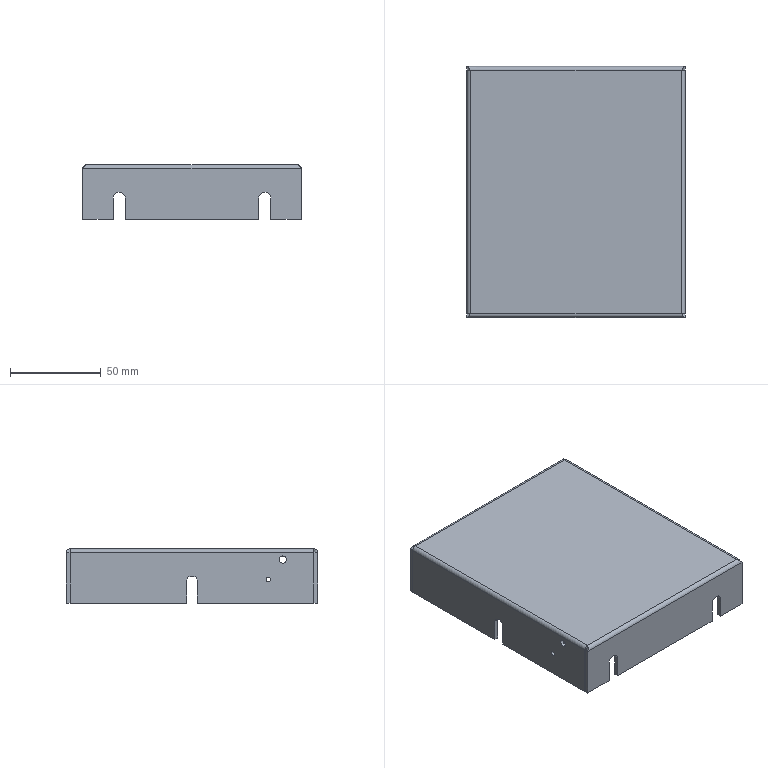Part | STEP file | communication module connection plate | 1 solid | 74 faces | box 120 x 138 x 30 mm | volume 59883 mm3 | plane 44 | cylinder 26 | spline 4 | commonest cylinder face diameters 6.6 x8 0.2 x4 2.5 x4 4 x4 4.2 x4 6 x2